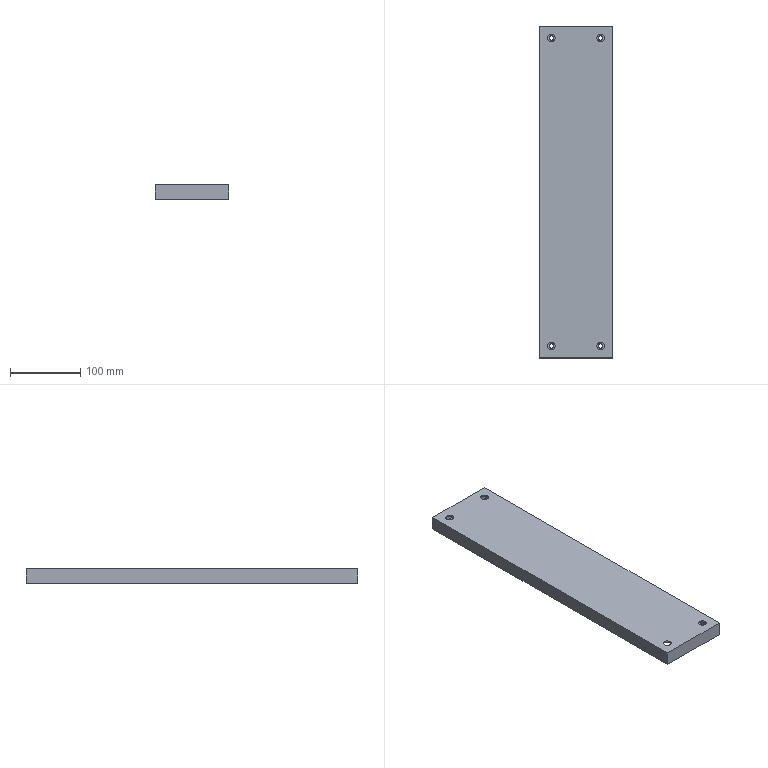Part | SolidWorks | features Extrusion 1, HoleWzd 1, ICE 1, Shell 1 | 1 solid | 32 faces | box 104 x 471 x 20 mm | volume 176278 mm3 | cylinder 16 | plane 16 | commonest cylinder face diameters 6.6 x8 11 x8
STEP:
#1=CARTESIAN_POINT('',(-38.3,218.5,0.));
#2=VERTEX_POINT('',#1);
#3=CARTESIAN_POINT('',(-31.7,218.5,0.));
#4=VERTEX_POINT('',#3);
#5=CARTESIAN_POINT('',(-35.,218.5,0.));
#6=DIRECTION('',(0.,0.,1.));
#7=DIRECTION('',(1.,0.,0.));
#8=AXIS2_PLACEMENT_3D('',#5,#6,#7);
#9=CIRCLE('',#8,3.3);
#10=EDGE_CURVE('',#2,#4,#9,.T.);
#11=ORIENTED_EDGE('',*,*,#10,.F.);
#12=CARTESIAN_POINT('',(-38.3,218.5,2.));
#13=VERTEX_POINT('',#12);
#14=CARTESIAN_POINT('',(-38.3,218.5,20.));
#15=DIRECTION('',(0.,0.,1.));
#16=VECTOR('',#15,1000.);
#17=LINE('',#14,#16);
#18=EDGE_CURVE('',#2,#13,#17,.T.);
#19=ORIENTED_EDGE('',*,*,#18,.T.);
#20=CARTESIAN_POINT('',(-31.7,218.5,2.));
#21=VERTEX_POINT('',#20);
#22=CARTESIAN_POINT('',(-35.,218.5,2.));
#23=DIRECTION('',(0.,0.,-1.));
#24=DIRECTION('',(-1.,0.,0.));
#25=AXIS2_PLACEMENT_3D('',#22,#23,#24);
#26=CIRCLE('',#25,3.3);
#27=EDGE_CURVE('',#21,#13,#26,.T.);
#28=ORIENTED_EDGE('',*,*,#27,.F.);
#29=CARTESIAN_POINT('',(-31.7,218.5,20.));
#30=DIRECTION('',(0.,0.,1.));
#31=VECTOR('',#30,1000.);
#32=LINE('',#29,#31);
#33=EDGE_CURVE('',#4,#21,#32,.T.);
#34=ORIENTED_EDGE('',*,*,#33,.F.);
#35=EDGE_LOOP('',(#11,#19,#28,#34));
#36=FACE_OUTER_BOUND('',#35,.T.);
#37=CARTESIAN_POINT('',(-35.,218.5,20.));
#38=DIRECTION('',(0.,0.,1.));
#39=DIRECTION('',(1.,0.,0.));
#40=AXIS2_PLACEMENT_3D('',#37,#38,#39);
#41=CYLINDRICAL_SURFACE('',#40,3.3);
#42=ADVANCED_FACE('',(#36),#41,.F.);
#43=CARTESIAN_POINT('',(-29.5,218.5,18.));
#44=VERTEX_POINT('',#43);
#45=CARTESIAN_POINT('',(-40.5,218.5,18.));
#46=VERTEX_POINT('',#45);
#47=CARTESIAN_POINT('',(-35.,218.5,18.));
#48=DIRECTION('',(0.,0.,-1.));
#49=DIRECTION('',(-1.,0.,0.));
#50=AXIS2_PLACEMENT_3D('',#47,#48,#49);
#51=CIRCLE('',#50,5.5);
#52=EDGE_CURVE('',#44,#46,#51,.T.);
#53=ORIENTED_EDGE('',*,*,#52,.T.);
#54=CARTESIAN_POINT('',(-40.5,218.5,20.));
#55=VERTEX_POINT('',#54);
#56=CARTESIAN_POINT('',(-40.5,218.5,20.));
#57=DIRECTION('',(0.,0.,1.));
#58=VECTOR('',#57,1000.);
#59=LINE('',#56,#58);
#60=EDGE_CURVE('',#46,#55,#59,.T.);
#61=ORIENTED_EDGE('',*,*,#60,.T.);
#62=CARTESIAN_POINT('',(-29.5,218.5,20.));
#63=VERTEX_POINT('',#62);
#64=CARTESIAN_POINT('',(-35.,218.5,20.));
#65=DIRECTION('',(0.,0.,1.));
#66=DIRECTION('',(1.,0.,0.));
#67=AXIS2_PLACEMENT_3D('',#64,#65,#66);
#68=CIRCLE('',#67,5.5);
#69=EDGE_CURVE('',#55,#63,#68,.T.);
#70=ORIENTED_EDGE('',*,*,#69,.T.);
#71=CARTESIAN_POINT('',(-29.5,218.5,20.));
#72=DIRECTION('',(0.,0.,1.));
#73=VECTOR('',#72,1000.);
#74=LINE('',#71,#73);
#75=EDGE_CURVE('',#44,#63,#74,.T.);
#76=ORIENTED_EDGE('',*,*,#75,.F.);
#77=EDGE_LOOP('',(#53,#61,#70,#76));
#78=FACE_OUTER_BOUND('',#77,.T.);
#79=CARTESIAN_POINT('',(-35.,218.5,20.));
#80=DIRECTION('',(0.,0.,1.));
#81=DIRECTION('',(1.,0.,0.));
#82=AXIS2_PLACEMENT_3D('',#79,#80,#81);
#83=CYLINDRICAL_SURFACE('',#82,5.5);
#84=ADVANCED_FACE('',(#78),#83,.F.);
#85=CARTESIAN_POINT('',(-29.5,-218.5,18.));
#86=VERTEX_POINT('',#85);
#87=CARTESIAN_POINT('',(-40.5,-218.5,18.));
#88=VERTEX_POINT('',#87);
#89=CARTESIAN_POINT('',(-35.,-218.5,18.));
#90=DIRECTION('',(0.,0.,-1.));
#91=DIRECTION('',(-1.,0.,0.));
#92=AXIS2_PLACEMENT_3D('',#89,#90,#91);
#93=CIRCLE('',#92,5.5);
#94=EDGE_CURVE('',#86,#88,#93,.T.);
#95=ORIENTED_EDGE('',*,*,#94,.T.);
#96=CARTESIAN_POINT('',(-40.5,-218.5,20.));
#97=VERTEX_POINT('',#96);
#98=CARTESIAN_POINT('',(-40.5,-218.5,20.));
#99=DIRECTION('',(0.,0.,1.));
#100=VECTOR('',#99,1000.);
#101=LINE('',#98,#100);
#102=EDGE_CURVE('',#88,#97,#101,.T.);
#103=ORIENTED_EDGE('',*,*,#102,.T.);
#104=CARTESIAN_POINT('',(-29.5,-218.5,20.));
#105=VERTEX_POINT('',#104);
#106=CARTESIAN_POINT('',(-35.,-218.5,20.));
#107=DIRECTION('',(0.,0.,1.));
#108=DIRECTION('',(1.,0.,0.));
#109=AXIS2_PLACEMENT_3D('',#106,#107,#108);
#110=CIRCLE('',#109,5.5);
#111=EDGE_CURVE('',#97,#105,#110,.T.);
#112=ORIENTED_EDGE('',*,*,#111,.T.);
#113=CARTESIAN_POINT('',(-29.5,-218.5,20.));
#114=DIRECTION('',(0.,0.,1.));
#115=VECTOR('',#114,1000.);
#116=LINE('',#113,#115);
#117=EDGE_CURVE('',#86,#105,#116,.T.);
#118=ORIENTED_EDGE('',*,*,#117,.F.);
#119=EDGE_LOOP('',(#95,#103,#112,#118));
#120=FACE_OUTER_BOUND('',#119,.T.);
#121=CARTESIAN_POINT('',(-35.,-218.5,20.));
#122=DIRECTION('',(0.,0.,1.));
#123=DIRECTION('',(1.,0.,0.));
#124=AXIS2_PLACEMENT_3D('',#121,#122,#123);
#125=CYLINDRICAL_SURFACE('',#124,5.5);
#126=ADVANCED_FACE('',(#120),#125,.F.);
#127=CARTESIAN_POINT('',(-38.3,-218.5,0.));
#128=VERTEX_POINT('',#127);
#129=CARTESIAN_POINT('',(-31.7,-218.5,0.));
#130=VERTEX_POINT('',#129);
#131=CARTESIAN_POINT('',(-35.,-218.5,0.));
#132=DIRECTION('',(0.,0.,1.));
#133=DIRECTION('',(1.,0.,0.));
#134=AXIS2_PLACEMENT_3D('',#131,#132,#133);
#135=CIRCLE('',#134,3.3);
#136=EDGE_CURVE('',#128,#130,#135,.T.);
#137=ORIENTED_EDGE('',*,*,#136,.F.);
#138=CARTESIAN_POINT('',(-38.3,-218.5,2.));
#139=VERTEX_POINT('',#138);
#140=CARTESIAN_POINT('',(-38.3,-218.5,20.));
#141=DIRECTION('',(0.,0.,1.));
#142=VECTOR('',#141,1000.);
#143=LINE('',#140,#142);
#144=EDGE_CURVE('',#128,#139,#143,.T.);
#145=ORIENTED_EDGE('',*,*,#144,.T.);
#146=CARTESIAN_POINT('',(-31.7,-218.5,2.));
#147=VERTEX_POINT('',#146);
#148=CARTESIAN_POINT('',(-35.,-218.5,2.));
#149=DIRECTION('',(0.,0.,-1.));
#150=DIRECTION('',(-1.,0.,0.));
#151=AXIS2_PLACEMENT_3D('',#148,#149,#150);
#152=CIRCLE('',#151,3.3);
#153=EDGE_CURVE('',#147,#139,#152,.T.);
#154=ORIENTED_EDGE('',*,*,#153,.F.);
#155=CARTESIAN_POINT('',(-31.7,-218.5,20.));
#156=DIRECTION('',(0.,0.,1.));
#157=VECTOR('',#156,1000.);
#158=LINE('',#155,#157);
#159=EDGE_CURVE('',#130,#147,#158,.T.);
#160=ORIENTED_EDGE('',*,*,#159,.F.);
#161=EDGE_LOOP('',(#137,#145,#154,#160));
#162=FACE_OUTER_BOUND('',#161,.T.);
#163=CARTESIAN_POINT('',(-35.,-218.5,20.));
#164=DIRECTION('',(0.,0.,1.));
#165=DIRECTION('',(1.,0.,0.));
#166=AXIS2_PLACEMENT_3D('',#163,#164,#165);
#167=CYLINDRICAL_SURFACE('',#166,3.3);
#168=ADVANCED_FACE('',(#162),#167,.F.);
#169=CARTESIAN_POINT('',(31.7,-218.5,0.));
#170=VERTEX_POINT('',#169);
#171=CARTESIAN_POINT('',(38.3,-218.5,0.));
#172=VERTEX_POINT('',#171);
#173=CARTESIAN_POINT('',(35.,-218.5,0.));
#174=DIRECTION('',(0.,0.,1.));
#175=DIRECTION('',(1.,0.,0.));
#176=AXIS2_PLACEMENT_3D('',#173,#174,#175);
#177=CIRCLE('',#176,3.3);
#178=EDGE_CURVE('',#170,#172,#177,.T.);
#179=ORIENTED_EDGE('',*,*,#178,.F.);
#180=CARTESIAN_POINT('',(31.7,-218.5,2.));
#181=VERTEX_POINT('',#180);
#182=CARTESIAN_POINT('',(31.7,-218.5,20.));
#183=DIRECTION('',(0.,0.,1.));
#184=VECTOR('',#183,1000.);
#185=LINE('',#182,#184);
#186=EDGE_CURVE('',#170,#181,#185,.T.);
#187=ORIENTED_EDGE('',*,*,#186,.T.);
#188=CARTESIAN_POINT('',(38.3,-218.5,2.));
#189=VERTEX_POINT('',#188);
#190=CARTESIAN_POINT('',(35.,-218.5,2.));
#191=DIRECTION('',(0.,0.,-1.));
#192=DIRECTION('',(-1.,0.,0.));
#193=AXIS2_PLACEMENT_3D('',#190,#191,#192);
#194=CIRCLE('',#193,3.3);
#195=EDGE_CURVE('',#189,#181,#194,.T.);
#196=ORIENTED_EDGE('',*,*,#195,.F.);
#197=CARTESIAN_POINT('',(38.3,-218.5,20.));
#198=DIRECTION('',(0.,0.,1.));
#199=VECTOR('',#198,1000.);
#200=LINE('',#197,#199);
#201=EDGE_CURVE('',#172,#189,#200,.T.);
#202=ORIENTED_EDGE('',*,*,#201,.F.);
#203=EDGE_LOOP('',(#179,#187,#196,#202));
#204=FACE_OUTER_BOUND('',#203,.T.);
#205=CARTESIAN_POINT('',(35.,-218.5,20.));
#206=DIRECTION('',(0.,0.,1.));
#207=DIRECTION('',(1.,0.,0.));
#208=AXIS2_PLACEMENT_3D('',#205,#206,#207);
#209=CYLINDRICAL_SURFACE('',#208,3.3);
#210=ADVANCED_FACE('',(#204),#209,.F.);
#211=CARTESIAN_POINT('',(40.5,-218.5,18.));
#212=VERTEX_POINT('',#211);
#213=CARTESIAN_POINT('',(29.5,-218.5,18.));
#214=VERTEX_POINT('',#213);
#215=CARTESIAN_POINT('',(35.,-218.5,18.));
#216=DIRECTION('',(0.,0.,-1.));
#217=DIRECTION('',(-1.,0.,0.));
#218=AXIS2_PLACEMENT_3D('',#215,#216,#217);
#219=CIRCLE('',#218,5.5);
#220=EDGE_CURVE('',#212,#214,#219,.T.);
#221=ORIENTED_EDGE('',*,*,#220,.T.);
#222=CARTESIAN_POINT('',(29.5,-218.5,20.));
#223=VERTEX_POINT('',#222);
#224=CARTESIAN_POINT('',(29.5,-218.5,20.));
#225=DIRECTION('',(0.,0.,1.));
#226=VECTOR('',#225,1000.);
#227=LINE('',#224,#226);
#228=EDGE_CURVE('',#214,#223,#227,.T.);
#229=ORIENTED_EDGE('',*,*,#228,.T.);
#230=CARTESIAN_POINT('',(40.5,-218.5,20.));
#231=VERTEX_POINT('',#230);
#232=CARTESIAN_POINT('',(35.,-218.5,20.));
#233=DIRECTION('',(0.,0.,1.));
#234=DIRECTION('',(1.,0.,0.));
#235=AXIS2_PLACEMENT_3D('',#232,#233,#234);
#236=CIRCLE('',#235,5.5);
#237=EDGE_CURVE('',#223,#231,#236,.T.);
#238=ORIENTED_EDGE('',*,*,#237,.T.);
#239=CARTESIAN_POINT('',(40.5,-218.5,20.));
#240=DIRECTION('',(0.,0.,1.));
#241=VECTOR('',#240,1000.);
#242=LINE('',#239,#241);
#243=EDGE_CURVE('',#212,#231,#242,.T.);
#244=ORIENTED_EDGE('',*,*,#243,.F.);
#245=EDGE_LOOP('',(#221,#229,#238,#244));
#246=FACE_OUTER_BOUND('',#245,.T.);
#247=CARTESIAN_POINT('',(35.,-218.5,20.));
#248=DIRECTION('',(0.,0.,1.));
#249=DIRECTION('',(1.,0.,0.));
#250=AXIS2_PLACEMENT_3D('',#247,#248,#249);
#251=CYLINDRICAL_SURFACE('',#250,5.5);
#252=ADVANCED_FACE('',(#246),#251,.F.);
#253=CARTESIAN_POINT('',(40.5,218.5,18.));
#254=VERTEX_POINT('',#253);
#255=CARTESIAN_POINT('',(29.5,218.5,18.));
#256=VERTEX_POINT('',#255);
#257=CARTESIAN_POINT('',(35.,218.5,18.));
#258=DIRECTION('',(0.,0.,-1.));
#259=DIRECTION('',(-1.,0.,0.));
#260=AXIS2_PLACEMENT_3D('',#257,#258,#259);
#261=CIRCLE('',#260,5.5);
#262=EDGE_CURVE('',#254,#256,#261,.T.);
#263=ORIENTED_EDGE('',*,*,#262,.T.);
#264=CARTESIAN_POINT('',(29.5,218.5,20.));
#265=VERTEX_POINT('',#264);
#266=CARTESIAN_POINT('',(29.5,218.5,20.));
#267=DIRECTION('',(0.,0.,1.));
#268=VECTOR('',#267,1000.);
#269=LINE('',#266,#268);
#270=EDGE_CURVE('',#256,#265,#269,.T.);
#271=ORIENTED_EDGE('',*,*,#270,.T.);
#272=CARTESIAN_POINT('',(40.5,218.5,20.));
#273=VERTEX_POINT('',#272);
#274=CARTESIAN_POINT('',(35.,218.5,20.));
#275=DIRECTION('',(0.,0.,1.));
#276=DIRECTION('',(1.,0.,0.));
#277=AXIS2_PLACEMENT_3D('',#274,#275,#276);
#278=CIRCLE('',#277,5.5);
#279=EDGE_CURVE('',#265,#273,#278,.T.);
#280=ORIENTED_EDGE('',*,*,#279,.T.);
#281=CARTESIAN_POINT('',(40.5,218.5,20.));
#282=DIRECTION('',(0.,0.,1.));
#283=VECTOR('',#282,1000.);
#284=LINE('',#281,#283);
#285=EDGE_CURVE('',#254,#273,#284,.T.);
#286=ORIENTED_EDGE('',*,*,#285,.F.);
#287=EDGE_LOOP('',(#263,#271,#280,#286));
#288=FACE_OUTER_BOUND('',#287,.T.);
#289=CARTESIAN_POINT('',(35.,218.5,20.));
#290=DIRECTION('',(0.,0.,1.));
#291=DIRECTION('',(1.,0.,0.));
#292=AXIS2_PLACEMENT_3D('',#289,#290,#291);
#293=CYLINDRICAL_SURFACE('',#292,5.5);
#294=ADVANCED_FACE('',(#288),#293,.F.);
#295=CARTESIAN_POINT('',(31.7,218.5,0.));
#296=VERTEX_POINT('',#295);
#297=CARTESIAN_POINT('',(38.3,218.5,0.));
#298=VERTEX_POINT('',#297);
#299=CARTESIAN_POINT('',(35.,218.5,0.));
#300=DIRECTION('',(0.,0.,1.));
#301=DIRECTION('',(1.,0.,0.));
#302=AXIS2_PLACEMENT_3D('',#299,#300,#301);
#303=CIRCLE('',#302,3.3);
#304=EDGE_CURVE('',#296,#298,#303,.T.);
#305=ORIENTED_EDGE('',*,*,#304,.F.);
#306=CARTESIAN_POINT('',(31.7,218.5,2.));
#307=VERTEX_POINT('',#306);
#308=CARTESIAN_POINT('',(31.7,218.5,20.));
#309=DIRECTION('',(0.,0.,1.));
#310=VECTOR('',#309,1000.);
#311=LINE('',#308,#310);
#312=EDGE_CURVE('',#296,#307,#311,.T.);
#313=ORIENTED_EDGE('',*,*,#312,.T.);
#314=CARTESIAN_POINT('',(38.3,218.5,2.));
#315=VERTEX_POINT('',#314);
#316=CARTESIAN_POINT('',(35.,218.5,2.));
#317=DIRECTION('',(0.,0.,-1.));
#318=DIRECTION('',(-1.,0.,0.));
#319=AXIS2_PLACEMENT_3D('',#316,#317,#318);
#320=CIRCLE('',#319,3.3);
#321=EDGE_CURVE('',#315,#307,#320,.T.);
#322=ORIENTED_EDGE('',*,*,#321,.F.);
#323=CARTESIAN_POINT('',(38.3,218.5,20.));
#324=DIRECTION('',(0.,0.,1.));
#325=VECTOR('',#324,1000.);
#326=LINE('',#323,#325);
#327=EDGE_CURVE('',#298,#315,#326,.T.);
#328=ORIENTED_EDGE('',*,*,#327,.F.);
#329=EDGE_LOOP('',(#305,#313,#322,#328));
#330=FACE_OUTER_BOUND('',#329,.T.);
#331=CARTESIAN_POINT('',(35.,218.5,20.));
#332=DIRECTION('',(0.,0.,1.));
#333=DIRECTION('',(1.,0.,0.));
#334=AXIS2_PLACEMENT_3D('',#331,#332,#333);
#335=CYLINDRICAL_SURFACE('',#334,3.3);
#336=ADVANCED_FACE('',(#330),#335,.F.);
#337=CARTESIAN_POINT('',(35.,-218.5,0.));
#338=DIRECTION('',(0.,0.,1.));
#339=DIRECTION('',(1.,0.,0.));
#340=AXIS2_PLACEMENT_3D('',#337,#338,#339);
#341=CIRCLE('',#340,3.3);
#342=EDGE_CURVE('',#172,#170,#341,.T.);
#343=ORIENTED_EDGE('',*,*,#342,.T.);
#344=ORIENTED_EDGE('',*,*,#178,.T.);
#345=EDGE_LOOP('',(#343,#344));
#346=FACE_BOUND('',#345,.T.);
#347=CARTESIAN_POINT('',(35.,218.5,0.));
#348=DIRECTION('',(0.,0.,1.));
#349=DIRECTION('',(1.,0.,0.));
#350=AXIS2_PLACEMENT_3D('',#347,#348,#349);
#351=CIRCLE('',#350,3.3);
#352=EDGE_CURVE('',#298,#296,#351,.T.);
#353=ORIENTED_EDGE('',*,*,#352,.T.);
#354=ORIENTED_EDGE('',*,*,#304,.T.);
#355=EDGE_LOOP('',(#353,#354));
#356=FACE_BOUND('',#355,.T.);
#357=CARTESIAN_POINT('',(52.,-235.5,0.));
#358=VERTEX_POINT('',#357);
#359=CARTESIAN_POINT('',(52.,235.5,0.));
#360=VERTEX_POINT('',#359);
#361=CARTESIAN_POINT('',(52.,-235.5,0.));
#362=DIRECTION('',(0.,1.,0.));
#363=VECTOR('',#362,1000.);
#364=LINE('',#361,#363);
#365=EDGE_CURVE('',#358,#360,#364,.T.);
#366=ORIENTED_EDGE('',*,*,#365,.F.);
#367=CARTESIAN_POINT('',(-52.,-235.5,0.));
#368=VERTEX_POINT('',#367);
#369=CARTESIAN_POINT('',(-52.,-235.5,0.));
#370=DIRECTION('',(1.,0.,0.));
#371=VECTOR('',#370,1000.);
#372=LINE('',#369,#371);
#373=EDGE_CURVE('',#368,#358,#372,.T.);
#374=ORIENTED_EDGE('',*,*,#373,.F.);
#375=CARTESIAN_POINT('',(-52.,235.5,0.));
#376=VERTEX_POINT('',#375);
#377=CARTESIAN_POINT('',(-52.,-235.5,0.));
#378=DIRECTION('',(0.,-1.,0.));
#379=VECTOR('',#378,1000.);
#380=LINE('',#377,#379);
#381=EDGE_CURVE('',#376,#368,#380,.T.);
#382=ORIENTED_EDGE('',*,*,#381,.F.);
#383=CARTESIAN_POINT('',(-52.,235.5,0.));
#384=DIRECTION('',(-1.,0.,0.));
#385=VECTOR('',#384,1000.);
#386=LINE('',#383,#385);
#387=EDGE_CURVE('',#360,#376,#386,.T.);
#388=ORIENTED_EDGE('',*,*,#387,.F.);
#389=EDGE_LOOP('',(#366,#374,#382,#388));
#390=FACE_OUTER_BOUND('',#389,.T.);
#391=CARTESIAN_POINT('',(32.,-215.5,0.));
#392=VERTEX_POINT('',#391);
#393=CARTESIAN_POINT('',(-32.,-215.5,0.));
#394=VERTEX_POINT('',#393);
#395=CARTESIAN_POINT('',(32.,-215.5,0.));
#396=DIRECTION('',(-1.,0.,0.));
#397=VECTOR('',#396,1000.);
#398=LINE('',#395,#397);
#399=EDGE_CURVE('',#392,#394,#398,.T.);
#400=ORIENTED_EDGE('',*,*,#399,.F.);
#401=CARTESIAN_POINT('',(32.,215.5,0.));
#402=VERTEX_POINT('',#401);
#403=CARTESIAN_POINT('',(32.,-215.5,0.));
#404=DIRECTION('',(0.,1.,0.));
#405=VECTOR('',#404,1000.);
#406=LINE('',#403,#405);
#407=EDGE_CURVE('',#392,#402,#406,.T.);
#408=ORIENTED_EDGE('',*,*,#407,.T.);
#409=CARTESIAN_POINT('',(-32.,215.5,0.));
#410=VERTEX_POINT('',#409);
#411=CARTESIAN_POINT('',(32.,215.5,0.));
#412=DIRECTION('',(-1.,0.,0.));
#413=VECTOR('',#412,1000.);
#414=LINE('',#411,#413);
#415=EDGE_CURVE('',#402,#410,#414,.T.);
#416=ORIENTED_EDGE('',*,*,#415,.T.);
#417=CARTESIAN_POINT('',(-32.,-215.5,0.));
#418=DIRECTION('',(0.,1.,0.));
#419=VECTOR('',#418,1000.);
#420=LINE('',#417,#419);
#421=EDGE_CURVE('',#394,#410,#420,.T.);
#422=ORIENTED_EDGE('',*,*,#421,.F.);
#423=EDGE_LOOP('',(#400,#408,#416,#422));
#424=FACE_BOUND('',#423,.T.);
#425=CARTESIAN_POINT('',(-35.,-218.5,0.));
#426=DIRECTION('',(0.,0.,1.));
#427=DIRECTION('',(1.,0.,0.));
#428=AXIS2_PLACEMENT_3D('',#425,#426,#427);
#429=CIRCLE('',#428,3.3);
#430=EDGE_CURVE('',#130,#128,#429,.T.);
#431=ORIENTED_EDGE('',*,*,#430,.T.);
#432=ORIENTED_EDGE('',*,*,#136,.T.);
#433=EDGE_LOOP('',(#431,#432));
#434=FACE_BOUND('',#433,.T.);
#435=CARTESIAN_POINT('',(-35.,218.5,0.));
#436=DIRECTION('',(0.,0.,1.));
#437=DIRECTION('',(1.,0.,0.));
#438=AXIS2_PLACEMENT_3D('',#435,#436,#437);
#439=CIRCLE('',#438,3.3);
#440=EDGE_CURVE('',#4,#2,#439,.T.);
#441=ORIENTED_EDGE('',*,*,#440,.T.);
#442=ORIENTED_EDGE('',*,*,#10,.T.);
#443=EDGE_LOOP('',(#441,#442));
#444=FACE_BOUND('',#443,.T.);
#445=CARTESIAN_POINT('',(0.,0.,0.));
#446=DIRECTION('',(0.,0.,-1.));
#447=DIRECTION('',(-1.,0.,0.));
#448=AXIS2_PLACEMENT_3D('',#445,#446,#447);
#449=PLANE('',#448);
#450=ADVANCED_FACE('',(#346,#356,#390,#424,#434,#444),#449,.T.);
#451=ORIENTED_EDGE('',*,*,#365,.T.);
#452=CARTESIAN_POINT('',(52.,235.5,20.));
#453=VERTEX_POINT('',#452);
#454=CARTESIAN_POINT('',(52.,235.5,20.));
#455=DIRECTION('',(0.,0.,-1.));
#456=VECTOR('',#455,1000.);
#457=LINE('',#454,#456);
#458=EDGE_CURVE('',#453,#360,#457,.T.);
#459=ORIENTED_EDGE('',*,*,#458,.F.);
#460=CARTESIAN_POINT('',(52.,-235.5,20.));
#461=VERTEX_POINT('',#460);
#462=CARTESIAN_POINT('',(52.,-235.5,20.));
#463=DIRECTION('',(0.,1.,0.));
#464=VECTOR('',#463,1000.);
#465=LINE('',#462,#464);
#466=EDGE_CURVE('',#461,#453,#465,.T.);
#467=ORIENTED_EDGE('',*,*,#466,.F.);
#468=CARTESIAN_POINT('',(52.,-235.5,20.));
#469=DIRECTION('',(0.,0.,-1.));
#470=VECTOR('',#469,1000.);
#471=LINE('',#468,#470);
#472=EDGE_CURVE('',#461,#358,#471,.T.);
#473=ORIENTED_EDGE('',*,*,#472,.T.);
#474=EDGE_LOOP('',(#451,#459,#467,#473));
#475=FACE_OUTER_BOUND('',#474,.T.);
#476=CARTESIAN_POINT('',(52.,-235.5,20.));
#477=DIRECTION('',(-1.,0.,0.));
#478=DIRECTION('',(0.,0.,1.));
#479=AXIS2_PLACEMENT_3D('',#476,#477,#478);
#480=PLANE('',#479);
#481=ADVANCED_FACE('',(#475),#480,.F.);
#482=ORIENTED_EDGE('',*,*,#387,.T.);
#483=CARTESIAN_POINT('',(-52.,235.5,20.));
#484=VERTEX_POINT('',#483);
#485=CARTESIAN_POINT('',(-52.,235.5,20.));
#486=DIRECTION('',(0.,0.,-1.));
#487=VECTOR('',#486,1000.);
#488=LINE('',#485,#487);
#489=EDGE_CURVE('',#484,#376,#488,.T.);
#490=ORIENTED_EDGE('',*,*,#489,.F.);
#491=CARTESIAN_POINT('',(-52.,235.5,20.));
#492=DIRECTION('',(-1.,0.,0.));
#493=VECTOR('',#492,1000.);
#494=LINE('',#491,#493);
#495=EDGE_CURVE('',#453,#484,#494,.T.);
#496=ORIENTED_EDGE('',*,*,#495,.F.);
#497=ORIENTED_EDGE('',*,*,#458,.T.);
#498=EDGE_LOOP('',(#482,#490,#496,#497));
#499=FACE_OUTER_BOUND('',#498,.T.);
#500=CARTESIAN_POINT('',(-52.,235.5,20.));
#501=DIRECTION('',(0.,-1.,0.));
#502=DIRECTION('',(0.,0.,-1.));
#503=AXIS2_PLACEMENT_3D('',#500,#501,#502);
#504=PLANE('',#503);
#505=ADVANCED_FACE('',(#499),#504,.F.);
#506=ORIENTED_EDGE('',*,*,#381,.T.);
#507=CARTESIAN_POINT('',(-52.,-235.5,20.));
#508=VERTEX_POINT('',#507);
#509=CARTESIAN_POINT('',(-52.,-235.5,20.));
#510=DIRECTION('',(0.,0.,-1.));
#511=VECTOR('',#510,1000.);
#512=LINE('',#509,#511);
#513=EDGE_CURVE('',#508,#368,#512,.T.);
#514=ORIENTED_EDGE('',*,*,#513,.F.);
#515=CARTESIAN_POINT('',(-52.,-235.5,20.));
#516=DIRECTION('',(0.,-1.,0.));
#517=VECTOR('',#516,1000.);
#518=LINE('',#515,#517);
#519=EDGE_CURVE('',#484,#508,#518,.T.);
#520=ORIENTED_EDGE('',*,*,#519,.F.);
#521=ORIENTED_EDGE('',*,*,#489,.T.);
#522=EDGE_LOOP('',(#506,#514,#520,#521));
#523=FACE_OUTER_BOUND('',#522,.T.);
#524=CARTESIAN_POINT('',(-52.,-235.5,20.));
#525=DIRECTION('',(1.,0.,0.));
#526=DIRECTION('',(0.,0.,-1.));
#527=AXIS2_PLACEMENT_3D('',#524,#525,#526);
#528=PLANE('',#527);
#529=ADVANCED_FACE('',(#523),#528,.F.);
#530=ORIENTED_EDGE('',*,*,#373,.T.);
#531=ORIENTED_EDGE('',*,*,#472,.F.);
#532=CARTESIAN_POINT('',(-52.,-235.5,20.));
#533=DIRECTION('',(1.,0.,0.));
#534=VECTOR('',#533,1000.);
#535=LINE('',#532,#534);
#536=EDGE_CURVE('',#508,#461,#535,.T.);
#537=ORIENTED_EDGE('',*,*,#536,.F.);
#538=ORIENTED_EDGE('',*,*,#513,.T.);
#539=EDGE_LOOP('',(#530,#531,#537,#538));
#540=FACE_OUTER_BOUND('',#539,.T.);
#541=CARTESIAN_POINT('',(-52.,-235.5,20.));
#542=DIRECTION('',(0.,1.,0.));
#543=DIRECTION('',(0.,0.,1.));
#544=AXIS2_PLACEMENT_3D('',#541,#542,#543);
#545=PLANE('',#544);
#546=ADVANCED_FACE('',(#540),#545,.F.);
#547=CARTESIAN_POINT('',(-35.,218.5,20.));
#548=DIRECTION('',(0.,0.,1.));
#549=DIRECTION('',(1.,0.,0.));
#550=AXIS2_PLACEMENT_3D('',#547,#548,#549);
#551=CIRCLE('',#550,5.5);
#552=EDGE_CURVE('',#63,#55,#551,.T.);
#553=ORIENTED_EDGE('',*,*,#552,.F.);
#554=ORIENTED_EDGE('',*,*,#69,.F.);
#555=EDGE_LOOP('',(#553,#554));
#556=FACE_BOUND('',#555,.T.);
#557=CARTESIAN_POINT('',(-35.,-218.5,20.));
#558=DIRECTION('',(0.,0.,1.));
#559=DIRECTION('',(1.,0.,0.));
#560=AXIS2_PLACEMENT_3D('',#557,#558,#559);
#561=CIRCLE('',#560,5.5);
#562=EDGE_CURVE('',#105,#97,#561,.T.);
#563=ORIENTED_EDGE('',*,*,#562,.F.);
#564=ORIENTED_EDGE('',*,*,#111,.F.);
#565=EDGE_LOOP('',(#563,#564));
#566=FACE_BOUND('',#565,.T.);
#567=CARTESIAN_POINT('',(35.,-218.5,20.));
#568=DIRECTION('',(0.,0.,1.));
#569=DIRECTION('',(1.,0.,0.));
#570=AXIS2_PLACEMENT_3D('',#567,#568,#569);
#571=CIRCLE('',#570,5.5);
#572=EDGE_CURVE('',#231,#223,#571,.T.);
#573=ORIENTED_EDGE('',*,*,#572,.F.);
#574=ORIENTED_EDGE('',*,*,#237,.F.);
#575=EDGE_LOOP('',(#573,#574));
#576=FACE_BOUND('',#575,.T.);
#577=CARTESIAN_POINT('',(35.,218.5,20.));
#578=DIRECTION('',(0.,0.,1.));
#579=DIRECTION('',(1.,0.,0.));
#580=AXIS2_PLACEMENT_3D('',#577,#578,#579);
#581=CIRCLE('',#580,5.5);
#582=EDGE_CURVE('',#273,#265,#581,.T.);
#583=ORIENTED_EDGE('',*,*,#582,.F.);
#584=ORIENTED_EDGE('',*,*,#279,.F.);
#585=EDGE_LOOP('',(#583,#584));
#586=FACE_BOUND('',#585,.T.);
#587=ORIENTED_EDGE('',*,*,#466,.T.);
#588=ORIENTED_EDGE('',*,*,#495,.T.);
#589=ORIENTED_EDGE('',*,*,#519,.T.);
#590=ORIENTED_EDGE('',*,*,#536,.T.);
#591=EDGE_LOOP('',(#587,#588,#589,#590));
#592=FACE_OUTER_BOUND('',#591,.T.);
#593=CARTESIAN_POINT('',(0.,0.,20.));
#594=DIRECTION('',(0.,0.,-1.));
#595=DIRECTION('',(-1.,0.,0.));
#596=AXIS2_PLACEMENT_3D('',#593,#594,#595);
#597=PLANE('',#596);
#598=ADVANCED_FACE('',(#556,#566,#576,#586,#592),#597,.F.);
#599=ORIENTED_EDGE('',*,*,#407,.F.);
#600=CARTESIAN_POINT('',(32.,-215.5,2.));
#601=VERTEX_POINT('',#600);
#602=CARTESIAN_POINT('',(32.,-215.5,2.));
#603=DIRECTION('',(0.,0.,-1.));
#604=VECTOR('',#603,1000.);
#605=LINE('',#602,#604);
#606=EDGE_CURVE('',#601,#392,#605,.T.);
#607=ORIENTED_EDGE('',*,*,#606,.F.);
#608=CARTESIAN_POINT('',(32.,215.5,2.));
#609=VERTEX_POINT('',#608);
#610=CARTESIAN_POINT('',(32.,-215.5,2.));
#611=DIRECTION('',(0.,1.,0.));
#612=VECTOR('',#611,1000.);
#613=LINE('',#610,#612);
#614=EDGE_CURVE('',#601,#609,#613,.T.);
#615=ORIENTED_EDGE('',*,*,#614,.T.);
#616=CARTESIAN_POINT('',(32.,215.5,2.));
#617=DIRECTION('',(0.,0.,-1.));
#618=VECTOR('',#617,1000.);
#619=LINE('',#616,#618);
#620=EDGE_CURVE('',#609,#402,#619,.T.);
#621=ORIENTED_EDGE('',*,*,#620,.T.);
#622=EDGE_LOOP('',(#599,#607,#615,#621));
#623=FACE_OUTER_BOUND('',#622,.T.);
#624=CARTESIAN_POINT('',(32.,-215.5,2.));
#625=DIRECTION('',(-1.,0.,0.));
#626=DIRECTION('',(0.,0.,1.));
#627=AXIS2_PLACEMENT_3D('',#624,#625,#626);
#628=PLANE('',#627);
#629=ADVANCED_FACE('',(#623),#628,.T.);
#630=ORIENTED_EDGE('',*,*,#415,.F.);
#631=ORIENTED_EDGE('',*,*,#620,.F.);
#632=CARTESIAN_POINT('',(-32.,215.5,2.));
#633=VERTEX_POINT('',#632);
#634=CARTESIAN_POINT('',(32.,215.5,2.));
#635=DIRECTION('',(-1.,0.,0.));
#636=VECTOR('',#635,1000.);
#637=LINE('',#634,#636);
#638=EDGE_CURVE('',#609,#633,#637,.T.);
#639=ORIENTED_EDGE('',*,*,#638,.T.);
#640=CARTESIAN_POINT('',(-32.,215.5,2.));
#641=DIRECTION('',(0.,0.,-1.));
#642=VECTOR('',#641,1000.);
#643=LINE('',#640,#642);
#644=EDGE_CURVE('',#633,#410,#643,.T.);
#645=ORIENTED_EDGE('',*,*,#644,.T.);
#646=EDGE_LOOP('',(#630,#631,#639,#645));
#647=FACE_OUTER_BOUND('',#646,.T.);
#648=CARTESIAN_POINT('',(32.,215.5,2.));
#649=DIRECTION('',(0.,-1.,0.));
#650=DIRECTION('',(0.,0.,-1.));
#651=AXIS2_PLACEMENT_3D('',#648,#649,#650);
#652=PLANE('',#651);
#653=ADVANCED_FACE('',(#647),#652,.T.);
#654=ORIENTED_EDGE('',*,*,#421,.T.);
#655=ORIENTED_EDGE('',*,*,#644,.F.);
#656=CARTESIAN_POINT('',(-32.,-215.5,2.));
#657=VERTEX_POINT('',#656);
#658=CARTESIAN_POINT('',(-32.,-215.5,2.));
#659=DIRECTION('',(0.,1.,0.));
#660=VECTOR('',#659,1000.);
#661=LINE('',#658,#660);
#662=EDGE_CURVE('',#657,#633,#661,.T.);
#663=ORIENTED_EDGE('',*,*,#662,.F.);
#664=CARTESIAN_POINT('',(-32.,-215.5,2.));
#665=DIRECTION('',(0.,0.,-1.));
#666=VECTOR('',#665,1000.);
#667=LINE('',#664,#666);
#668=EDGE_CURVE('',#657,#394,#667,.T.);
#669=ORIENTED_EDGE('',*,*,#668,.T.);
#670=EDGE_LOOP('',(#654,#655,#663,#669));
#671=FACE_OUTER_BOUND('',#670,.T.);
#672=CARTESIAN_POINT('',(-32.,-215.5,2.));
#673=DIRECTION('',(-1.,0.,0.));
#674=DIRECTION('',(0.,0.,1.));
#675=AXIS2_PLACEMENT_3D('',#672,#673,#674);
#676=PLANE('',#675);
#677=ADVANCED_FACE('',(#671),#676,.F.);
#678=ORIENTED_EDGE('',*,*,#399,.T.);
#679=ORIENTED_EDGE('',*,*,#668,.F.);
#680=CARTESIAN_POINT('',(32.,-215.5,2.));
#681=DIRECTION('',(-1.,0.,0.));
#682=VECTOR('',#681,1000.);
#683=LINE('',#680,#682);
#684=EDGE_CURVE('',#601,#657,#683,.T.);
#685=ORIENTED_EDGE('',*,*,#684,.F.);
#686=ORIENTED_EDGE('',*,*,#606,.T.);
#687=EDGE_LOOP('',(#678,#679,#685,#686));
#688=FACE_OUTER_BOUND('',#687,.T.);
#689=CARTESIAN_POINT('',(32.,-215.5,2.));
#690=DIRECTION('',(0.,-1.,0.));
#691=DIRECTION('',(0.,0.,-1.));
#692=AXIS2_PLACEMENT_3D('',#689,#690,#691);
#693=PLANE('',#692);
#694=ADVANCED_FACE('',(#688),#693,.F.);
#695=ORIENTED_EDGE('',*,*,#27,.T.);
#696=CARTESIAN_POINT('',(-35.,218.5,2.));
#697=DIRECTION('',(0.,0.,-1.));
#698=DIRECTION('',(-1.,0.,0.));
#699=AXIS2_PLACEMENT_3D('',#696,#697,#698);
#700=CIRCLE('',#699,3.3);
#701=EDGE_CURVE('',#13,#21,#700,.T.);
#702=ORIENTED_EDGE('',*,*,#701,.T.);
#703=EDGE_LOOP('',(#695,#702));
#704=FACE_BOUND('',#703,.T.);
#705=ORIENTED_EDGE('',*,*,#153,.T.);
#706=CARTESIAN_POINT('',(-35.,-218.5,2.));
#707=DIRECTION('',(0.,0.,-1.));
#708=DIRECTION('',(-1.,0.,0.));
#709=AXIS2_PLACEMENT_3D('',#706,#707,#708);
#710=CIRCLE('',#709,3.3);
#711=EDGE_CURVE('',#139,#147,#710,.T.);
#712=ORIENTED_EDGE('',*,*,#711,.T.);
#713=EDGE_LOOP('',(#705,#712));
#714=FACE_BOUND('',#713,.T.);
#715=ORIENTED_EDGE('',*,*,#195,.T.);
#716=CARTESIAN_POINT('',(35.,-218.5,2.));
#717=DIRECTION('',(0.,0.,-1.));
#718=DIRECTION('',(-1.,0.,0.));
#719=AXIS2_PLACEMENT_3D('',#716,#717,#718);
#720=CIRCLE('',#719,3.3);
#721=EDGE_CURVE('',#181,#189,#720,.T.);
#722=ORIENTED_EDGE('',*,*,#721,.T.);
#723=EDGE_LOOP('',(#715,#722));
#724=FACE_BOUND('',#723,.T.);
#725=ORIENTED_EDGE('',*,*,#321,.T.);
#726=CARTESIAN_POINT('',(35.,218.5,2.));
#727=DIRECTION('',(0.,0.,-1.));
#728=DIRECTION('',(-1.,0.,0.));
#729=AXIS2_PLACEMENT_3D('',#726,#727,#728);
#730=CIRCLE('',#729,3.3);
#731=EDGE_CURVE('',#307,#315,#730,.T.);
#732=ORIENTED_EDGE('',*,*,#731,.T.);
#733=EDGE_LOOP('',(#725,#732));
#734=FACE_BOUND('',#733,.T.);
#735=CARTESIAN_POINT('',(50.,-233.5,2.));
#736=VERTEX_POINT('',#735);
#737=CARTESIAN_POINT('',(50.,233.5,2.));
#738=VERTEX_POINT('',#737);
#739=CARTESIAN_POINT('',(50.,0.,2.));
#740=DIRECTION('',(0.,1.,0.));
#741=VECTOR('',#740,1000.);
#742=LINE('',#739,#741);
#743=EDGE_CURVE('',#736,#738,#742,.T.);
#744=ORIENTED_EDGE('',*,*,#743,.T.);
#745=CARTESIAN_POINT('',(-50.,233.5,2.));
#746=VERTEX_POINT('',#745);
#747=CARTESIAN_POINT('',(0.,233.5,2.));
#748=DIRECTION('',(-1.,0.,0.));
#749=VECTOR('',#748,1000.);
#750=LINE('',#747,#749);
#751=EDGE_CURVE('',#738,#746,#750,.T.);
#752=ORIENTED_EDGE('',*,*,#751,.T.);
#753=CARTESIAN_POINT('',(-50.,-233.5,2.));
#754=VERTEX_POINT('',#753);
#755=CARTESIAN_POINT('',(-50.,0.,2.));
#756=DIRECTION('',(0.,-1.,0.));
#757=VECTOR('',#756,1000.);
#758=LINE('',#755,#757);
#759=EDGE_CURVE('',#746,#754,#758,.T.);
#760=ORIENTED_EDGE('',*,*,#759,.T.);
#761=CARTESIAN_POINT('',(0.,-233.5,2.));
#762=DIRECTION('',(1.,0.,0.));
#763=VECTOR('',#762,1000.);
#764=LINE('',#761,#763);
#765=EDGE_CURVE('',#754,#736,#764,.T.);
#766=ORIENTED_EDGE('',*,*,#765,.T.);
#767=EDGE_LOOP('',(#744,#752,#760,#766));
#768=FACE_OUTER_BOUND('',#767,.T.);
#769=ORIENTED_EDGE('',*,*,#684,.T.);
#770=ORIENTED_EDGE('',*,*,#662,.T.);
#771=ORIENTED_EDGE('',*,*,#638,.F.);
#772=ORIENTED_EDGE('',*,*,#614,.F.);
#773=EDGE_LOOP('',(#769,#770,#771,#772));
#774=FACE_BOUND('',#773,.T.);
#775=CARTESIAN_POINT('',(0.,0.,2.));
#776=DIRECTION('',(0.,0.,-1.));
#777=DIRECTION('',(-1.,0.,0.));
#778=AXIS2_PLACEMENT_3D('',#775,#776,#777);
#779=PLANE('',#778);
#780=ADVANCED_FACE('',(#704,#714,#724,#734,#768,#774),#779,.F.);
#781=ORIENTED_EDGE('',*,*,#743,.F.);
#782=CARTESIAN_POINT('',(50.,-233.5,18.));
#783=VERTEX_POINT('',#782);
#784=CARTESIAN_POINT('',(50.,-233.5,20.));
#785=DIRECTION('',(0.,0.,-1.));
#786=VECTOR('',#785,1000.);
#787=LINE('',#784,#786);
#788=EDGE_CURVE('',#783,#736,#787,.T.);
#789=ORIENTED_EDGE('',*,*,#788,.F.);
#790=CARTESIAN_POINT('',(50.,233.5,18.));
#791=VERTEX_POINT('',#790);
#792=CARTESIAN_POINT('',(50.,0.,18.));
#793=DIRECTION('',(0.,1.,0.));
#794=VECTOR('',#793,1000.);
#795=LINE('',#792,#794);
#796=EDGE_CURVE('',#783,#791,#795,.T.);
#797=ORIENTED_EDGE('',*,*,#796,.T.);
#798=CARTESIAN_POINT('',(50.,233.5,20.));
#799=DIRECTION('',(0.,0.,-1.));
#800=VECTOR('',#799,1000.);
#801=LINE('',#798,#800);
#802=EDGE_CURVE('',#791,#738,#801,.T.);
#803=ORIENTED_EDGE('',*,*,#802,.T.);
#804=EDGE_LOOP('',(#781,#789,#797,#803));
#805=FACE_OUTER_BOUND('',#804,.T.);
#806=CARTESIAN_POINT('',(50.,-235.5,20.));
#807=DIRECTION('',(-1.,0.,0.));
#808=DIRECTION('',(0.,0.,1.));
#809=AXIS2_PLACEMENT_3D('',#806,#807,#808);
#810=PLANE('',#809);
#811=ADVANCED_FACE('',(#805),#810,.T.);
#812=ORIENTED_EDGE('',*,*,#751,.F.);
#813=ORIENTED_EDGE('',*,*,#802,.F.);
#814=CARTESIAN_POINT('',(-50.,233.5,18.));
#815=VERTEX_POINT('',#814);
#816=CARTESIAN_POINT('',(0.,233.5,18.));
#817=DIRECTION('',(-1.,0.,0.));
#818=VECTOR('',#817,1000.);
#819=LINE('',#816,#818);
#820=EDGE_CURVE('',#791,#815,#819,.T.);
#821=ORIENTED_EDGE('',*,*,#820,.T.);
#822=CARTESIAN_POINT('',(-50.,233.5,20.));
#823=DIRECTION('',(0.,0.,-1.));
#824=VECTOR('',#823,1000.);
#825=LINE('',#822,#824);
#826=EDGE_CURVE('',#815,#746,#825,.T.);
#827=ORIENTED_EDGE('',*,*,#826,.T.);
#828=EDGE_LOOP('',(#812,#813,#821,#827));
#829=FACE_OUTER_BOUND('',#828,.T.);
#830=CARTESIAN_POINT('',(-52.,233.5,20.));
#831=DIRECTION('',(0.,-1.,0.));
#832=DIRECTION('',(0.,0.,-1.));
#833=AXIS2_PLACEMENT_3D('',#830,#831,#832);
#834=PLANE('',#833);
#835=ADVANCED_FACE('',(#829),#834,.T.);
#836=ORIENTED_EDGE('',*,*,#759,.F.);
#837=ORIENTED_EDGE('',*,*,#826,.F.);
#838=CARTESIAN_POINT('',(-50.,-233.5,18.));
#839=VERTEX_POINT('',#838);
#840=CARTESIAN_POINT('',(-50.,0.,18.));
#841=DIRECTION('',(0.,-1.,0.));
#842=VECTOR('',#841,1000.);
#843=LINE('',#840,#842);
#844=EDGE_CURVE('',#815,#839,#843,.T.);
#845=ORIENTED_EDGE('',*,*,#844,.T.);
#846=CARTESIAN_POINT('',(-50.,-233.5,20.));
#847=DIRECTION('',(0.,0.,-1.));
#848=VECTOR('',#847,1000.);
#849=LINE('',#846,#848);
#850=EDGE_CURVE('',#839,#754,#849,.T.);
#851=ORIENTED_EDGE('',*,*,#850,.T.);
#852=EDGE_LOOP('',(#836,#837,#845,#851));
#853=FACE_OUTER_BOUND('',#852,.T.);
#854=CARTESIAN_POINT('',(-50.,-235.5,20.));
#855=DIRECTION('',(1.,0.,0.));
#856=DIRECTION('',(0.,0.,-1.));
#857=AXIS2_PLACEMENT_3D('',#854,#855,#856);
#858=PLANE('',#857);
#859=ADVANCED_FACE('',(#853),#858,.T.);
#860=ORIENTED_EDGE('',*,*,#765,.F.);
#861=ORIENTED_EDGE('',*,*,#850,.F.);
#862=CARTESIAN_POINT('',(0.,-233.5,18.));
#863=DIRECTION('',(1.,0.,0.));
#864=VECTOR('',#863,1000.);
#865=LINE('',#862,#864);
#866=EDGE_CURVE('',#839,#783,#865,.T.);
#867=ORIENTED_EDGE('',*,*,#866,.T.);
#868=ORIENTED_EDGE('',*,*,#788,.T.);
#869=EDGE_LOOP('',(#860,#861,#867,#868));
#870=FACE_OUTER_BOUND('',#869,.T.);
#871=CARTESIAN_POINT('',(-52.,-233.5,20.));
#872=DIRECTION('',(0.,1.,0.));
#873=DIRECTION('',(0.,0.,1.));
#874=AXIS2_PLACEMENT_3D('',#871,#872,#873);
#875=PLANE('',#874);
#876=ADVANCED_FACE('',(#870),#875,.T.);
#877=ORIENTED_EDGE('',*,*,#52,.F.);
#878=CARTESIAN_POINT('',(-35.,218.5,18.));
#879=DIRECTION('',(0.,0.,-1.));
#880=DIRECTION('',(-1.,0.,0.));
#881=AXIS2_PLACEMENT_3D('',#878,#879,#880);
#882=CIRCLE('',#881,5.5);
#883=EDGE_CURVE('',#46,#44,#882,.T.);
#884=ORIENTED_EDGE('',*,*,#883,.F.);
#885=EDGE_LOOP('',(#877,#884));
#886=FACE_BOUND('',#885,.T.);
#887=ORIENTED_EDGE('',*,*,#94,.F.);
#888=CARTESIAN_POINT('',(-35.,-218.5,18.));
#889=DIRECTION('',(0.,0.,-1.));
#890=DIRECTION('',(-1.,0.,0.));
#891=AXIS2_PLACEMENT_3D('',#888,#889,#890);
#892=CIRCLE('',#891,5.5);
#893=EDGE_CURVE('',#88,#86,#892,.T.);
#894=ORIENTED_EDGE('',*,*,#893,.F.);
#895=EDGE_LOOP('',(#887,#894));
#896=FACE_BOUND('',#895,.T.);
#897=ORIENTED_EDGE('',*,*,#220,.F.);
#898=CARTESIAN_POINT('',(35.,-218.5,18.));
#899=DIRECTION('',(0.,0.,-1.));
#900=DIRECTION('',(-1.,0.,0.));
#901=AXIS2_PLACEMENT_3D('',#898,#899,#900);
#902=CIRCLE('',#901,5.5);
#903=EDGE_CURVE('',#214,#212,#902,.T.);
#904=ORIENTED_EDGE('',*,*,#903,.F.);
#905=EDGE_LOOP('',(#897,#904));
#906=FACE_BOUND('',#905,.T.);
#907=ORIENTED_EDGE('',*,*,#262,.F.);
#908=CARTESIAN_POINT('',(35.,218.5,18.));
#909=DIRECTION('',(0.,0.,-1.));
#910=DIRECTION('',(-1.,0.,0.));
#911=AXIS2_PLACEMENT_3D('',#908,#909,#910);
#912=CIRCLE('',#911,5.5);
#913=EDGE_CURVE('',#256,#254,#912,.T.);
#914=ORIENTED_EDGE('',*,*,#913,.F.);
#915=EDGE_LOOP('',(#907,#914));
#916=FACE_BOUND('',#915,.T.);
#917=ORIENTED_EDGE('',*,*,#796,.F.);
#918=ORIENTED_EDGE('',*,*,#866,.F.);
#919=ORIENTED_EDGE('',*,*,#844,.F.);
#920=ORIENTED_EDGE('',*,*,#820,.F.);
#921=EDGE_LOOP('',(#917,#918,#919,#920));
#922=FACE_OUTER_BOUND('',#921,.T.);
#923=CARTESIAN_POINT('',(0.,0.,18.));
#924=DIRECTION('',(0.,0.,-1.));
#925=DIRECTION('',(-1.,0.,0.));
#926=AXIS2_PLACEMENT_3D('',#923,#924,#925);
#927=PLANE('',#926);
#928=ADVANCED_FACE('',(#886,#896,#906,#916,#922),#927,.T.);
#929=ORIENTED_EDGE('',*,*,#312,.F.);
#930=ORIENTED_EDGE('',*,*,#352,.F.);
#931=ORIENTED_EDGE('',*,*,#327,.T.);
#932=ORIENTED_EDGE('',*,*,#731,.F.);
#933=EDGE_LOOP('',(#929,#930,#931,#932));
#934=FACE_OUTER_BOUND('',#933,.T.);
#935=CARTESIAN_POINT('',(35.,218.5,20.));
#936=DIRECTION('',(0.,0.,1.));
#937=DIRECTION('',(1.,0.,0.));
#938=AXIS2_PLACEMENT_3D('',#935,#936,#937);
#939=CYLINDRICAL_SURFACE('',#938,3.3);
#940=ADVANCED_FACE('',(#934),#939,.F.);
#941=ORIENTED_EDGE('',*,*,#270,.F.);
#942=ORIENTED_EDGE('',*,*,#913,.T.);
#943=ORIENTED_EDGE('',*,*,#285,.T.);
#944=ORIENTED_EDGE('',*,*,#582,.T.);
#945=EDGE_LOOP('',(#941,#942,#943,#944));
#946=FACE_OUTER_BOUND('',#945,.T.);
#947=CARTESIAN_POINT('',(35.,218.5,20.));
#948=DIRECTION('',(0.,0.,1.));
#949=DIRECTION('',(1.,0.,0.));
#950=AXIS2_PLACEMENT_3D('',#947,#948,#949);
#951=CYLINDRICAL_SURFACE('',#950,5.5);
#952=ADVANCED_FACE('',(#946),#951,.F.);
#953=ORIENTED_EDGE('',*,*,#228,.F.);
#954=ORIENTED_EDGE('',*,*,#903,.T.);
#955=ORIENTED_EDGE('',*,*,#243,.T.);
#956=ORIENTED_EDGE('',*,*,#572,.T.);
#957=EDGE_LOOP('',(#953,#954,#955,#956));
#958=FACE_OUTER_BOUND('',#957,.T.);
#959=CARTESIAN_POINT('',(35.,-218.5,20.));
#960=DIRECTION('',(0.,0.,1.));
#961=DIRECTION('',(1.,0.,0.));
#962=AXIS2_PLACEMENT_3D('',#959,#960,#961);
#963=CYLINDRICAL_SURFACE('',#962,5.5);
#964=ADVANCED_FACE('',(#958),#963,.F.);
#965=ORIENTED_EDGE('',*,*,#186,.F.);
#966=ORIENTED_EDGE('',*,*,#342,.F.);
#967=ORIENTED_EDGE('',*,*,#201,.T.);
#968=ORIENTED_EDGE('',*,*,#721,.F.);
#969=EDGE_LOOP('',(#965,#966,#967,#968));
#970=FACE_OUTER_BOUND('',#969,.T.);
#971=CARTESIAN_POINT('',(35.,-218.5,20.));
#972=DIRECTION('',(0.,0.,1.));
#973=DIRECTION('',(1.,0.,0.));
#974=AXIS2_PLACEMENT_3D('',#971,#972,#973);
#975=CYLINDRICAL_SURFACE('',#974,3.3);
#976=ADVANCED_FACE('',(#970),#975,.F.);
#977=ORIENTED_EDGE('',*,*,#144,.F.);
#978=ORIENTED_EDGE('',*,*,#430,.F.);
#979=ORIENTED_EDGE('',*,*,#159,.T.);
#980=ORIENTED_EDGE('',*,*,#711,.F.);
#981=EDGE_LOOP('',(#977,#978,#979,#980));
#982=FACE_OUTER_BOUND('',#981,.T.);
#983=CARTESIAN_POINT('',(-35.,-218.5,20.));
#984=DIRECTION('',(0.,0.,1.));
#985=DIRECTION('',(1.,0.,0.));
#986=AXIS2_PLACEMENT_3D('',#983,#984,#985);
#987=CYLINDRICAL_SURFACE('',#986,3.3);
#988=ADVANCED_FACE('',(#982),#987,.F.);
#989=ORIENTED_EDGE('',*,*,#102,.F.);
#990=ORIENTED_EDGE('',*,*,#893,.T.);
#991=ORIENTED_EDGE('',*,*,#117,.T.);
#992=ORIENTED_EDGE('',*,*,#562,.T.);
#993=EDGE_LOOP('',(#989,#990,#991,#992));
#994=FACE_OUTER_BOUND('',#993,.T.);
#995=CARTESIAN_POINT('',(-35.,-218.5,20.));
#996=DIRECTION('',(0.,0.,1.));
#997=DIRECTION('',(1.,0.,0.));
#998=AXIS2_PLACEMENT_3D('',#995,#996,#997);
#999=CYLINDRICAL_SURFACE('',#998,5.5);
#1000=ADVANCED_FACE('',(#994),#999,.F.);
#1001=ORIENTED_EDGE('',*,*,#60,.F.);
#1002=ORIENTED_EDGE('',*,*,#883,.T.);
#1003=ORIENTED_EDGE('',*,*,#75,.T.);
#1004=ORIENTED_EDGE('',*,*,#552,.T.);
#1005=EDGE_LOOP('',(#1001,#1002,#1003,#1004));
#1006=FACE_OUTER_BOUND('',#1005,.T.);
#1007=CARTESIAN_POINT('',(-35.,218.5,20.));
#1008=DIRECTION('',(0.,0.,1.));
#1009=DIRECTION('',(1.,0.,0.));
#1010=AXIS2_PLACEMENT_3D('',#1007,#1008,#1009);
#1011=CYLINDRICAL_SURFACE('',#1010,5.5);
#1012=ADVANCED_FACE('',(#1006),#1011,.F.);
#1013=ORIENTED_EDGE('',*,*,#18,.F.);
#1014=ORIENTED_EDGE('',*,*,#440,.F.);
#1015=ORIENTED_EDGE('',*,*,#33,.T.);
#1016=ORIENTED_EDGE('',*,*,#701,.F.);
#1017=EDGE_LOOP('',(#1013,#1014,#1015,#1016));
#1018=FACE_OUTER_BOUND('',#1017,.T.);
#1019=CARTESIAN_POINT('',(-35.,218.5,20.));
#1020=DIRECTION('',(0.,0.,1.));
#1021=DIRECTION('',(1.,0.,0.));
#1022=AXIS2_PLACEMENT_3D('',#1019,#1020,#1021);
#1023=CYLINDRICAL_SURFACE('',#1022,3.3);
#1024=ADVANCED_FACE('',(#1018),#1023,.F.);
#1025=CLOSED_SHELL('',(#42,#84,#126,#168,#210,#252,#294,#336,#450,#481,#505,#529,#546,#598,#629,#653,#677,#694,#780,#811,#835,#859,#876,#928,#940,#952,#964,#976,#988,#1000,#1012,#1024));
#1026=MANIFOLD_SOLID_BREP('',#1025);
#1027=CARTESIAN_POINT('',(0.,0.,0.));
#1028=DIRECTION('',(0.,0.,1.));
#1029=DIRECTION('',(1.,0.,0.));
#1030=AXIS2_PLACEMENT_3D('',#1027,#1028,#1029);
#1031=(LENGTH_UNIT()NAMED_UNIT(*)SI_UNIT(.MILLI.,.METRE.));
#1032=UNCERTAINTY_MEASURE_WITH_UNIT(LENGTH_MEASURE(0.00001),#1031,'','');
#1033=(NAMED_UNIT(*)PLANE_ANGLE_UNIT()SI_UNIT($,.RADIAN.));
#1034=(NAMED_UNIT(*)SI_UNIT($,.STERADIAN.)SOLID_ANGLE_UNIT());
#1035=(GEOMETRIC_REPRESENTATION_CONTEXT(3)GLOBAL_UNCERTAINTY_ASSIGNED_CONTEXT((#1032))GLOBAL_UNIT_ASSIGNED_CONTEXT((#1031,#1033,#1034))REPRESENTATION_CONTEXT('',''));
#1036=ADVANCED_BREP_SHAPE_REPRESENTATION('',(#1026,#1030),#1035);